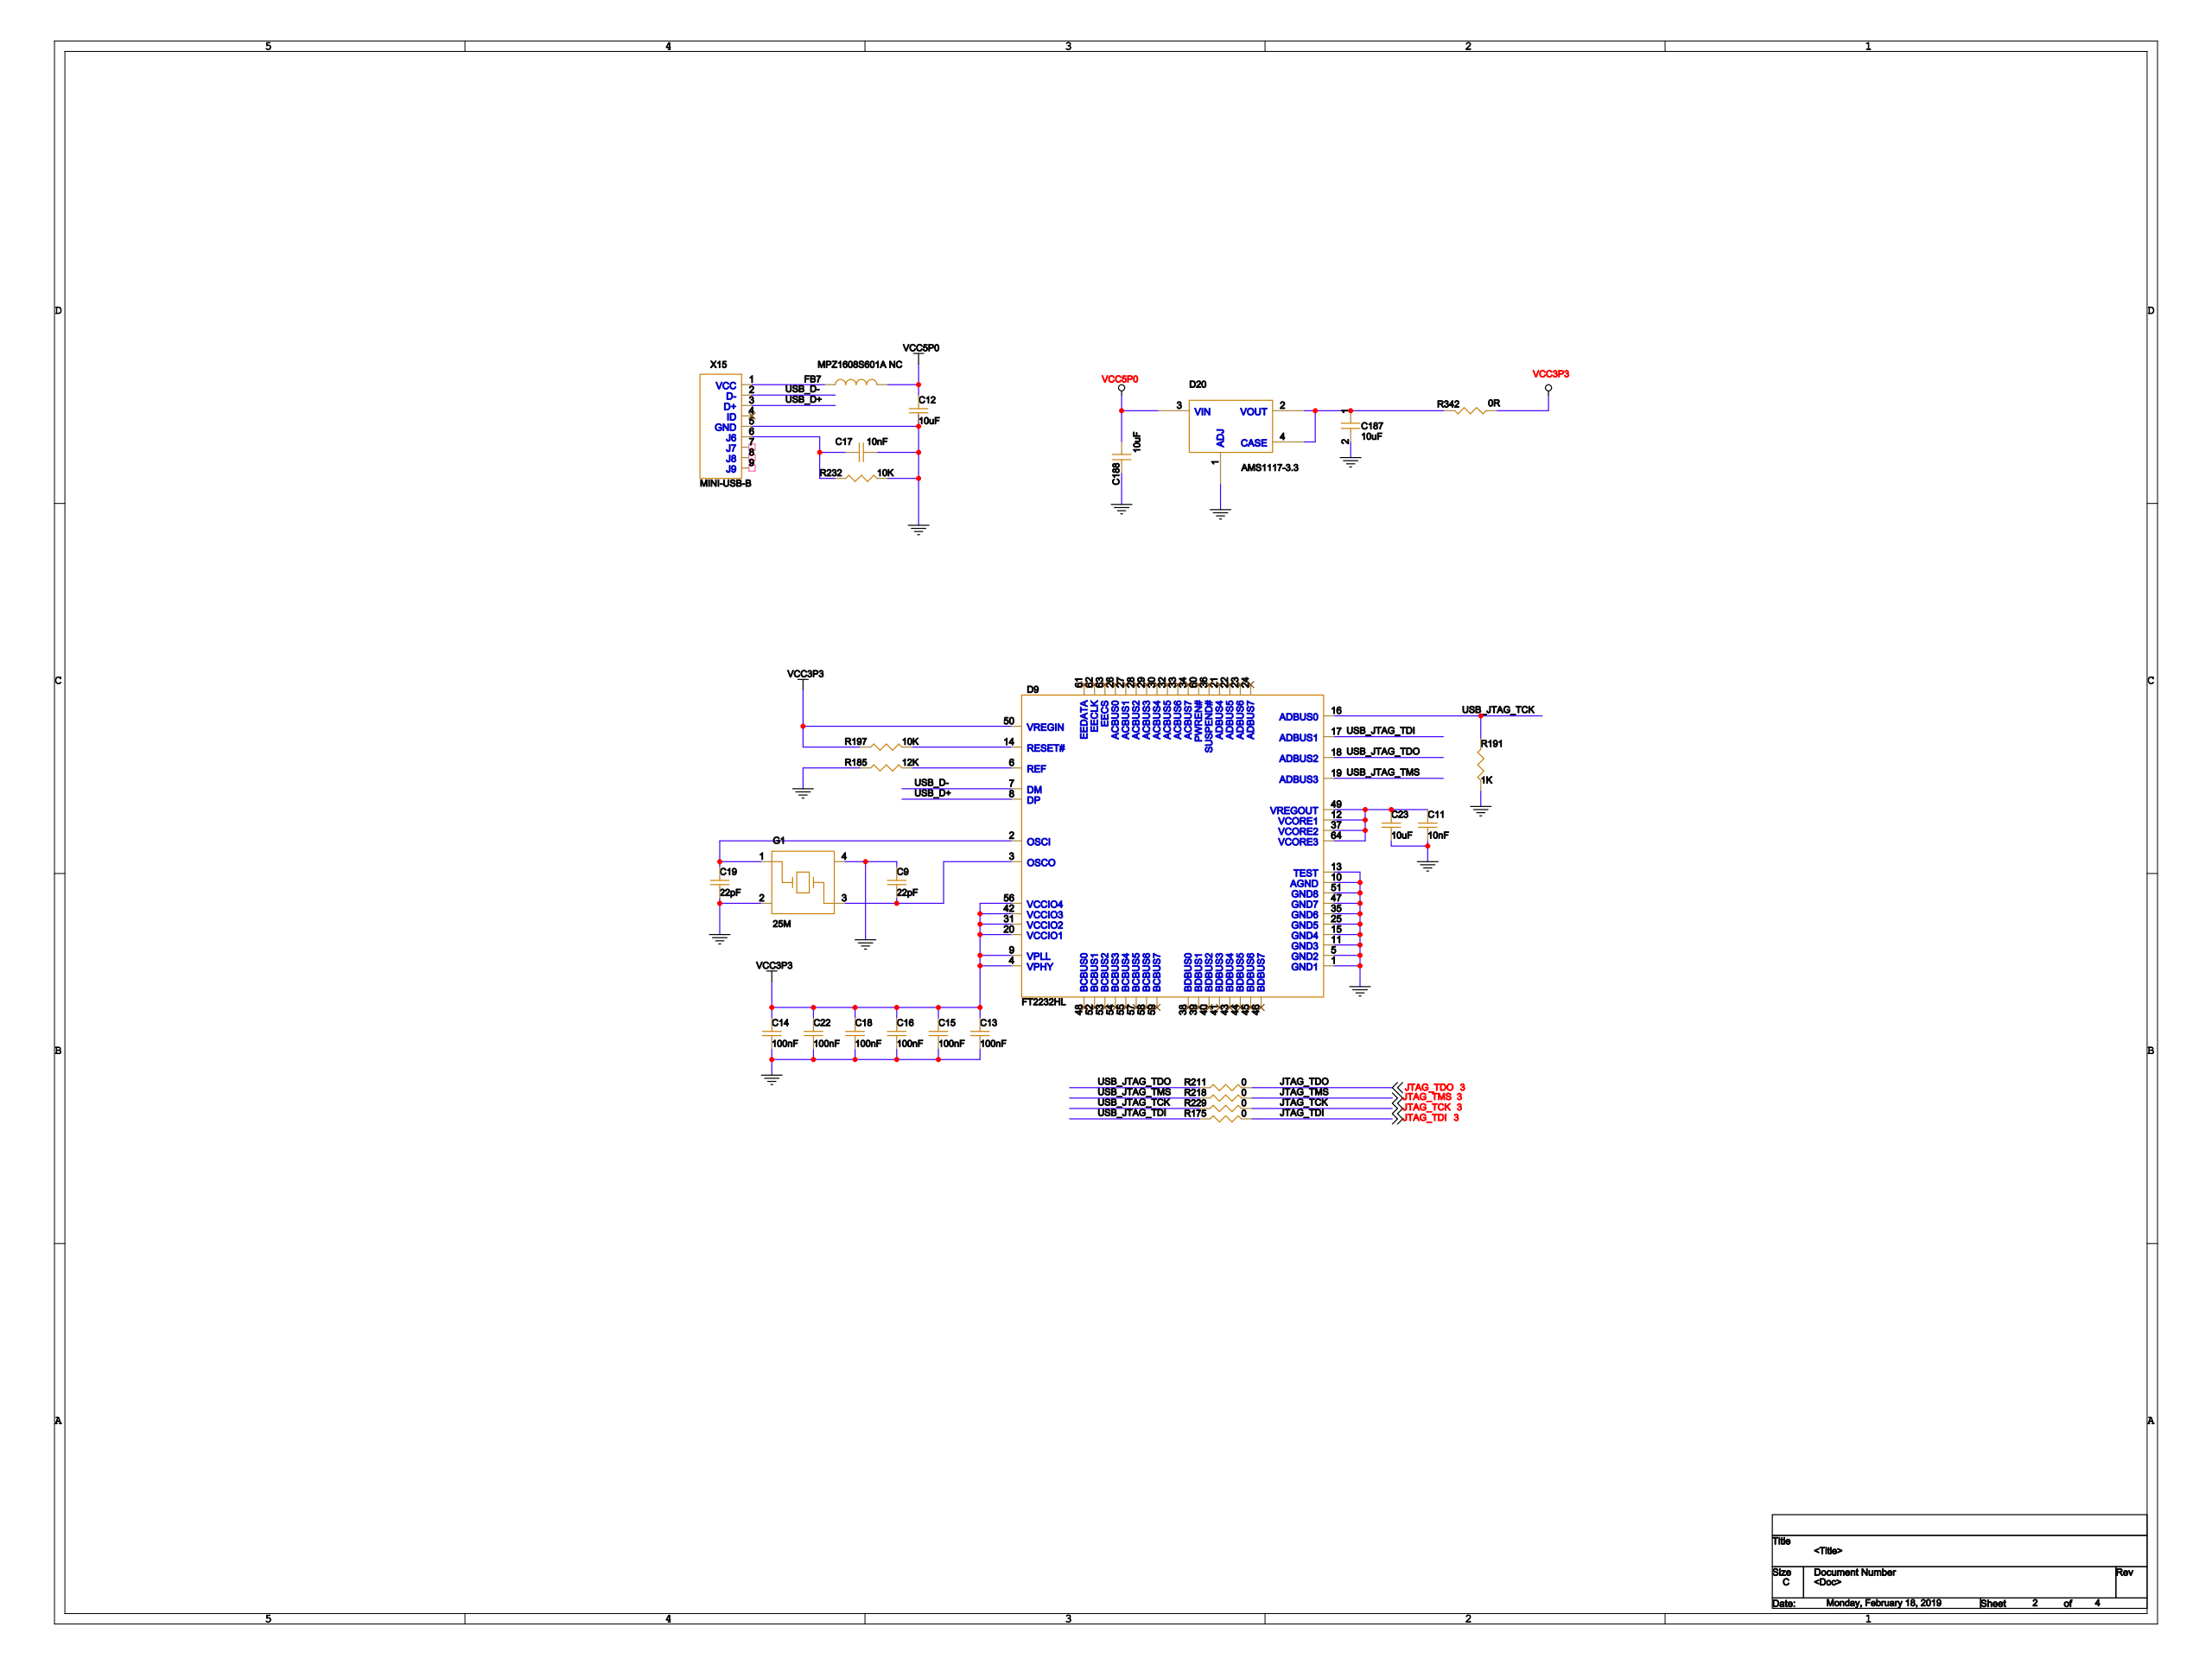Circuit board | Cadence Allegro | 174 parts | 250 nets | one sheet of the schematic
Parts on this sheet (reference | value | footprint):
C9 | 22pF | SMC0603
C11 | 10nF | SMC0603
C12 | 10uF | C0805
C13 | 100nF | SMC0603
C14 | 100nF | SMC0603
C15 | 100nF | SMC0603
C16 | 100nF | SMC0603
C17 | 10nF | SMC0603
C18 | 100nF | SMC0603
C19 | 22pF | SMC0603
C22 | 100nF | SMC0603
C23 | 10uF | C0805
C187 | 10uF | C0805
C188 | 10uF | C0805
D9 | FT2232HL | LQFP64_D12_E12_P0R5
D20 | AMS1117-3.3 | SOT-223
FB7 | MPZ1608S601A NC | FB0603
G1 | 25M | RA5032
R175 | 0 | R0603
R185 | 12K | R0603
R191 | 1K | R0603
R197 | 10K | R0603
R211 | 0 | R0603
R218 | 0 | R0603
R229 | 0 | R0603
R232 | 10K | R0603
R342 | 0R | R0603
X15 | MINI-USB-B | MINIUSBB
Nets of these parts (net: part-pin ...):
N2533401: C11-1 C23-1 D9-12 D9-37 D9-49 D9-64
GND: C9-1 C11-2 C12-2 C13-2 C14-2 C15-2 C16-2 C17-2 C18-2 C19-2 C22-2 C23-2 C187-2 C188-2 D20-1 G1-2 G1-4 R185-1 R191-1 R232-2 X15-5 D9-1 D9-5 D9-10 D9-11 D9-13 D9-15 D9-25 D9-35 D9-47 D9-51
N2533917: C17-1 R232-1 X15-6
VCC3P3: C13-1 C14-1 C15-1 C16-1 C18-1 C22-1 R197-1 R342-1 D9-4 D9-9 D9-20 D9-31 D9-42 D9-50 D9-56
N2533019: C19-1 G1-1 D9-2
N2533051: C9-2 G1-3 D9-3
VCC5P0: C12-1 C188-1 D20-3 FB7-2
N2535413: C187-1 D20-2 D20-4 R342-2
JTAG_TMS: R218-2
JTAG_TCK: R229-2
JTAG_TDI: R175-2
JTAG_TDO: R211-2
USB_JTAG_TCK: R191-2 R229-1 D9-16
USB_JTAG_TDI: R175-1 D9-17
USB_JTAG_TDO: R211-1 D9-18
USB_JTAG_TMS: R218-1 D9-19
USB_D-: X15-2 D9-7
USB_D+: X15-3 D9-8
N2532991: R185-2 D9-6
N2532947: R197-2 D9-14
N2533643: FB7-1 X15-1